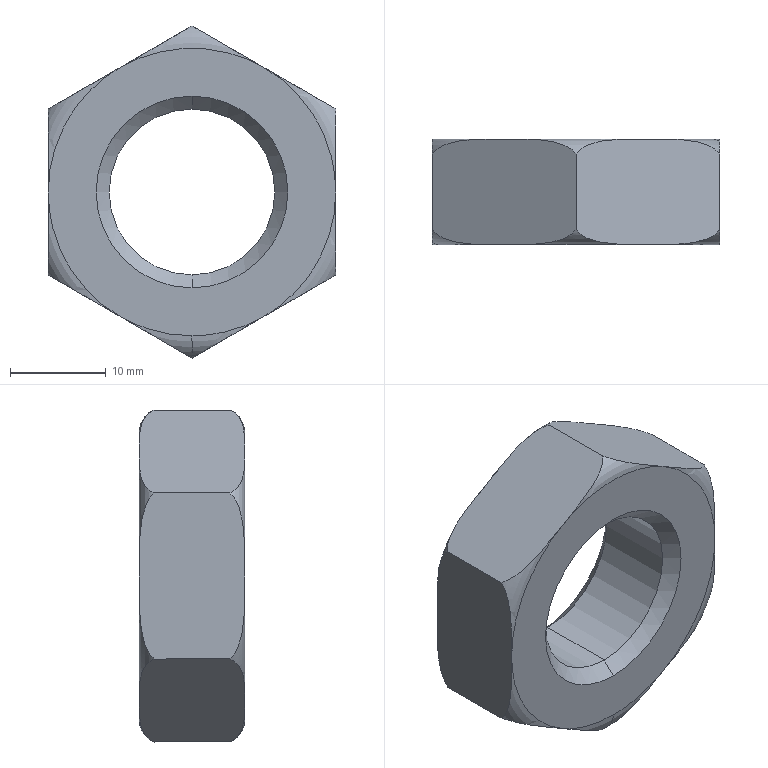Part | SolidWorks | features BaseBody 1 | 1 solid | 28 faces | box 30 x 11 x 34.641 mm | volume 5813 mm3 | torus 14 | plane 8 | cone 4 | cylinder 2 | commonest cylinder face diameters 17.294 x2